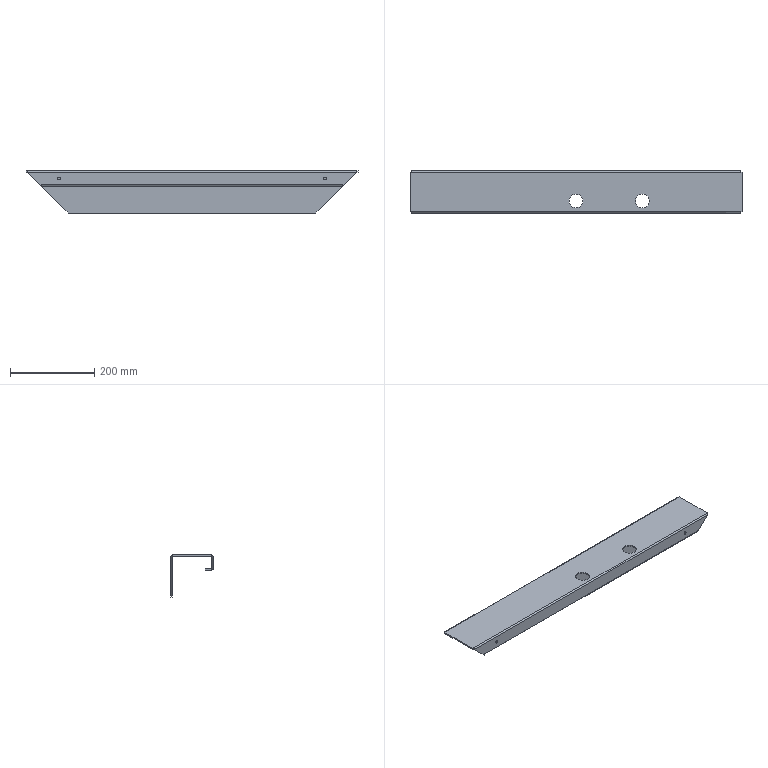Part | STEP file | HESS-408-70-15W-W-12-bottom frame 2 | 1 solid | 66 faces | box 790 x 100 x 100 mm | volume 531868 mm3 | plane 32 | cylinder 30 | spline 4 | commonest cylinder face diameters 3.2 x12 6.8 x4 33 x4 40 x4 0.2 x3 6.2 x3